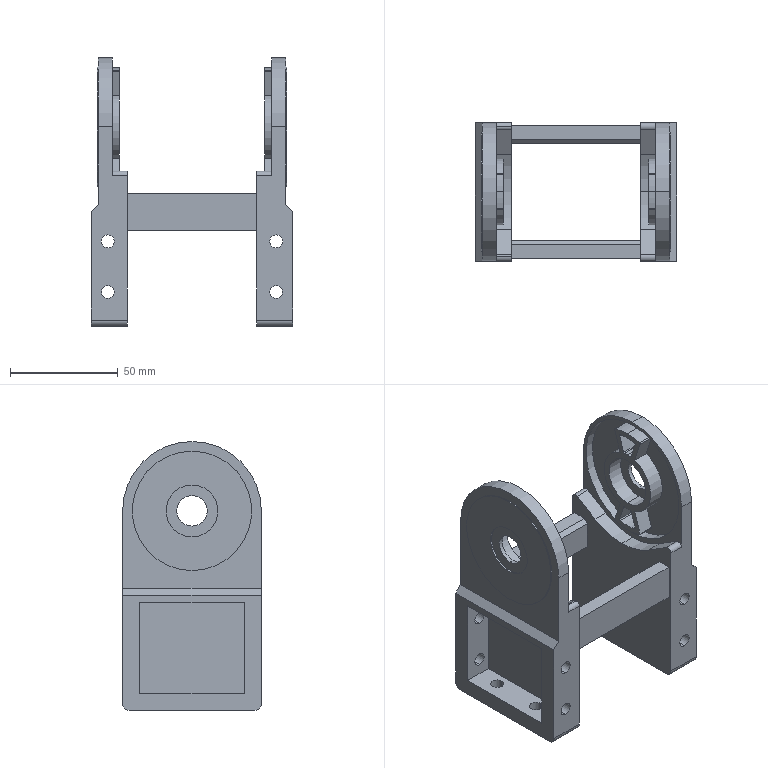Part | SolidWorks | features BaseBody 1 | 1 solid | 182 faces | box 93.538 x 64.35 x 124.74 mm | volume 121596 mm3 | cylinder 110 | plane 72 | commonest cylinder face diameters 1 x24 6 x24 24 x8 4 x6 49.578 x6 54.608 x6